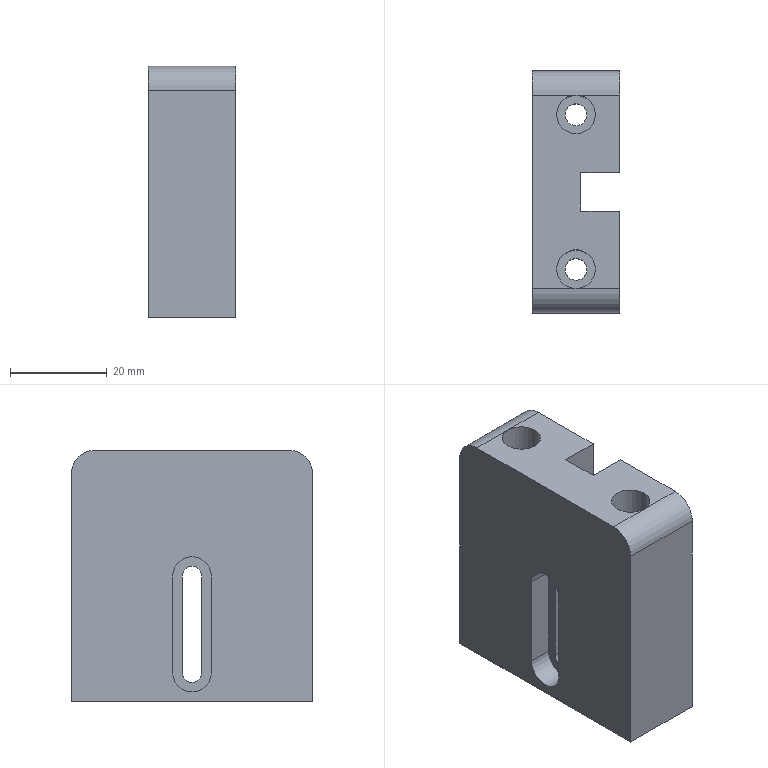Part | SolidWorks | features ICE 2, Extrusion 1, Fillet 1, HoleWzd 1 | 1 solid | 31 faces | box 18 x 50 x 52 mm | volume 37362 mm3 | plane 17 | cylinder 14 | commonest cylinder face diameters 8 x6 4.5 x4 4 x2 10 x2
STEP:
#1=CARTESIAN_POINT('',(-4.,16.,12.));
#2=VERTEX_POINT('',#1);
#3=CARTESIAN_POINT('',(4.,16.,12.));
#4=VERTEX_POINT('',#3);
#5=CARTESIAN_POINT('',(0.,16.,12.));
#6=DIRECTION('',(0.,0.,1.));
#7=DIRECTION('',(1.,0.,0.));
#8=AXIS2_PLACEMENT_3D('',#5,#6,#7);
#9=CIRCLE('',#8,4.);
#10=EDGE_CURVE('',#2,#4,#9,.T.);
#11=ORIENTED_EDGE('',*,*,#10,.F.);
#12=CARTESIAN_POINT('',(-4.,16.,52.));
#13=VERTEX_POINT('',#12);
#14=CARTESIAN_POINT('',(-4.,16.,52.));
#15=DIRECTION('',(0.,0.,1.));
#16=VECTOR('',#15,1000.);
#17=LINE('',#14,#16);
#18=EDGE_CURVE('',#2,#13,#17,.T.);
#19=ORIENTED_EDGE('',*,*,#18,.T.);
#20=CARTESIAN_POINT('',(4.,16.,52.));
#21=VERTEX_POINT('',#20);
#22=CARTESIAN_POINT('',(0.,16.,52.));
#23=DIRECTION('',(0.,0.,1.));
#24=DIRECTION('',(1.,0.,0.));
#25=AXIS2_PLACEMENT_3D('',#22,#23,#24);
#26=CIRCLE('',#25,4.);
#27=EDGE_CURVE('',#13,#21,#26,.T.);
#28=ORIENTED_EDGE('',*,*,#27,.T.);
#29=CARTESIAN_POINT('',(4.,16.,52.));
#30=DIRECTION('',(0.,0.,1.));
#31=VECTOR('',#30,1000.);
#32=LINE('',#29,#31);
#33=EDGE_CURVE('',#4,#21,#32,.T.);
#34=ORIENTED_EDGE('',*,*,#33,.F.);
#35=EDGE_LOOP('',(#11,#19,#28,#34));
#36=FACE_OUTER_BOUND('',#35,.T.);
#37=CARTESIAN_POINT('',(0.,16.,52.));
#38=DIRECTION('',(0.,0.,1.));
#39=DIRECTION('',(1.,0.,0.));
#40=AXIS2_PLACEMENT_3D('',#37,#38,#39);
#41=CYLINDRICAL_SURFACE('',#40,4.);
#42=ADVANCED_FACE('',(#36),#41,.F.);
#43=CARTESIAN_POINT('',(-2.25,16.,0.));
#44=VERTEX_POINT('',#43);
#45=CARTESIAN_POINT('',(2.25,16.,0.));
#46=VERTEX_POINT('',#45);
#47=CARTESIAN_POINT('',(0.,16.,0.));
#48=DIRECTION('',(0.,0.,1.));
#49=DIRECTION('',(1.,0.,0.));
#50=AXIS2_PLACEMENT_3D('',#47,#48,#49);
#51=CIRCLE('',#50,2.25);
#52=EDGE_CURVE('',#44,#46,#51,.T.);
#53=ORIENTED_EDGE('',*,*,#52,.F.);
#54=CARTESIAN_POINT('',(-2.25,16.,12.));
#55=VERTEX_POINT('',#54);
#56=CARTESIAN_POINT('',(-2.25,16.,52.));
#57=DIRECTION('',(0.,0.,1.));
#58=VECTOR('',#57,1000.);
#59=LINE('',#56,#58);
#60=EDGE_CURVE('',#44,#55,#59,.T.);
#61=ORIENTED_EDGE('',*,*,#60,.T.);
#62=CARTESIAN_POINT('',(2.25,16.,12.));
#63=VERTEX_POINT('',#62);
#64=CARTESIAN_POINT('',(0.,16.,12.));
#65=DIRECTION('',(0.,0.,1.));
#66=DIRECTION('',(1.,0.,0.));
#67=AXIS2_PLACEMENT_3D('',#64,#65,#66);
#68=CIRCLE('',#67,2.25);
#69=EDGE_CURVE('',#55,#63,#68,.T.);
#70=ORIENTED_EDGE('',*,*,#69,.T.);
#71=CARTESIAN_POINT('',(2.25,16.,52.));
#72=DIRECTION('',(0.,0.,1.));
#73=VECTOR('',#72,1000.);
#74=LINE('',#71,#73);
#75=EDGE_CURVE('',#46,#63,#74,.T.);
#76=ORIENTED_EDGE('',*,*,#75,.F.);
#77=EDGE_LOOP('',(#53,#61,#70,#76));
#78=FACE_OUTER_BOUND('',#77,.T.);
#79=CARTESIAN_POINT('',(0.,16.,52.));
#80=DIRECTION('',(0.,0.,1.));
#81=DIRECTION('',(1.,0.,0.));
#82=AXIS2_PLACEMENT_3D('',#79,#80,#81);
#83=CYLINDRICAL_SURFACE('',#82,2.25);
#84=ADVANCED_FACE('',(#78),#83,.F.);
#85=CARTESIAN_POINT('',(-4.,-16.,12.));
#86=VERTEX_POINT('',#85);
#87=CARTESIAN_POINT('',(4.,-16.,12.));
#88=VERTEX_POINT('',#87);
#89=CARTESIAN_POINT('',(0.,-16.,12.));
#90=DIRECTION('',(0.,0.,1.));
#91=DIRECTION('',(1.,0.,0.));
#92=AXIS2_PLACEMENT_3D('',#89,#90,#91);
#93=CIRCLE('',#92,4.);
#94=EDGE_CURVE('',#86,#88,#93,.T.);
#95=ORIENTED_EDGE('',*,*,#94,.F.);
#96=CARTESIAN_POINT('',(-4.,-16.,52.));
#97=VERTEX_POINT('',#96);
#98=CARTESIAN_POINT('',(-4.,-16.,52.));
#99=DIRECTION('',(0.,0.,1.));
#100=VECTOR('',#99,1000.);
#101=LINE('',#98,#100);
#102=EDGE_CURVE('',#86,#97,#101,.T.);
#103=ORIENTED_EDGE('',*,*,#102,.T.);
#104=CARTESIAN_POINT('',(0.,-20.,52.));
#105=VERTEX_POINT('',#104);
#106=CARTESIAN_POINT('',(0.,-16.,52.));
#107=DIRECTION('',(0.,0.,1.));
#108=DIRECTION('',(1.,0.,0.));
#109=AXIS2_PLACEMENT_3D('',#106,#107,#108);
#110=CIRCLE('',#109,4.);
#111=EDGE_CURVE('',#97,#105,#110,.T.);
#112=ORIENTED_EDGE('',*,*,#111,.T.);
#113=CARTESIAN_POINT('',(4.,-16.,52.));
#114=VERTEX_POINT('',#113);
#115=CARTESIAN_POINT('',(0.,-16.,52.));
#116=DIRECTION('',(0.,0.,1.));
#117=DIRECTION('',(1.,0.,0.));
#118=AXIS2_PLACEMENT_3D('',#115,#116,#117);
#119=CIRCLE('',#118,4.);
#120=EDGE_CURVE('',#105,#114,#119,.T.);
#121=ORIENTED_EDGE('',*,*,#120,.T.);
#122=CARTESIAN_POINT('',(4.,-16.,52.));
#123=DIRECTION('',(0.,0.,1.));
#124=VECTOR('',#123,1000.);
#125=LINE('',#122,#124);
#126=EDGE_CURVE('',#88,#114,#125,.T.);
#127=ORIENTED_EDGE('',*,*,#126,.F.);
#128=EDGE_LOOP('',(#95,#103,#112,#121,#127));
#129=FACE_OUTER_BOUND('',#128,.T.);
#130=CARTESIAN_POINT('',(0.,-16.,52.));
#131=DIRECTION('',(0.,0.,1.));
#132=DIRECTION('',(1.,0.,0.));
#133=AXIS2_PLACEMENT_3D('',#130,#131,#132);
#134=CYLINDRICAL_SURFACE('',#133,4.);
#135=ADVANCED_FACE('',(#129),#134,.F.);
#136=CARTESIAN_POINT('',(-2.25,-16.,0.));
#137=VERTEX_POINT('',#136);
#138=CARTESIAN_POINT('',(2.25,-16.,0.));
#139=VERTEX_POINT('',#138);
#140=CARTESIAN_POINT('',(0.,-16.,0.));
#141=DIRECTION('',(0.,0.,1.));
#142=DIRECTION('',(1.,0.,0.));
#143=AXIS2_PLACEMENT_3D('',#140,#141,#142);
#144=CIRCLE('',#143,2.25);
#145=EDGE_CURVE('',#137,#139,#144,.T.);
#146=ORIENTED_EDGE('',*,*,#145,.F.);
#147=CARTESIAN_POINT('',(-2.25,-16.,12.));
#148=VERTEX_POINT('',#147);
#149=CARTESIAN_POINT('',(-2.25,-16.,52.));
#150=DIRECTION('',(0.,0.,1.));
#151=VECTOR('',#150,1000.);
#152=LINE('',#149,#151);
#153=EDGE_CURVE('',#137,#148,#152,.T.);
#154=ORIENTED_EDGE('',*,*,#153,.T.);
#155=CARTESIAN_POINT('',(2.25,-16.,12.));
#156=VERTEX_POINT('',#155);
#157=CARTESIAN_POINT('',(0.,-16.,12.));
#158=DIRECTION('',(0.,0.,1.));
#159=DIRECTION('',(1.,0.,0.));
#160=AXIS2_PLACEMENT_3D('',#157,#158,#159);
#161=CIRCLE('',#160,2.25);
#162=EDGE_CURVE('',#148,#156,#161,.T.);
#163=ORIENTED_EDGE('',*,*,#162,.T.);
#164=CARTESIAN_POINT('',(2.25,-16.,52.));
#165=DIRECTION('',(0.,0.,1.));
#166=VECTOR('',#165,1000.);
#167=LINE('',#164,#166);
#168=EDGE_CURVE('',#139,#156,#167,.T.);
#169=ORIENTED_EDGE('',*,*,#168,.F.);
#170=EDGE_LOOP('',(#146,#154,#163,#169));
#171=FACE_OUTER_BOUND('',#170,.T.);
#172=CARTESIAN_POINT('',(0.,-16.,52.));
#173=DIRECTION('',(0.,0.,1.));
#174=DIRECTION('',(1.,0.,0.));
#175=AXIS2_PLACEMENT_3D('',#172,#173,#174);
#176=CYLINDRICAL_SURFACE('',#175,2.25);
#177=ADVANCED_FACE('',(#171),#176,.F.);
#178=CARTESIAN_POINT('',(9.,-25.,47.));
#179=VERTEX_POINT('',#178);
#180=CARTESIAN_POINT('',(9.,-25.,0.));
#181=VERTEX_POINT('',#180);
#182=CARTESIAN_POINT('',(9.,-25.,52.));
#183=DIRECTION('',(0.,0.,-1.));
#184=VECTOR('',#183,1000.);
#185=LINE('',#182,#184);
#186=EDGE_CURVE('',#179,#181,#185,.T.);
#187=ORIENTED_EDGE('',*,*,#186,.F.);
#188=CARTESIAN_POINT('',(-9.,-25.,47.));
#189=VERTEX_POINT('',#188);
#190=CARTESIAN_POINT('',(-9.,-25.,47.));
#191=DIRECTION('',(-1.,0.,0.));
#192=VECTOR('',#191,1000.);
#193=LINE('',#190,#192);
#194=EDGE_CURVE('',#179,#189,#193,.T.);
#195=ORIENTED_EDGE('',*,*,#194,.T.);
#196=CARTESIAN_POINT('',(-9.,-25.,0.));
#197=VERTEX_POINT('',#196);
#198=CARTESIAN_POINT('',(-9.,-25.,52.));
#199=DIRECTION('',(0.,0.,-1.));
#200=VECTOR('',#199,1000.);
#201=LINE('',#198,#200);
#202=EDGE_CURVE('',#189,#197,#201,.T.);
#203=ORIENTED_EDGE('',*,*,#202,.T.);
#204=CARTESIAN_POINT('',(-9.,-25.,0.));
#205=DIRECTION('',(1.,0.,0.));
#206=VECTOR('',#205,1000.);
#207=LINE('',#204,#206);
#208=EDGE_CURVE('',#197,#181,#207,.T.);
#209=ORIENTED_EDGE('',*,*,#208,.T.);
#210=EDGE_LOOP('',(#187,#195,#203,#209));
#211=FACE_OUTER_BOUND('',#210,.T.);
#212=CARTESIAN_POINT('',(-9.,-25.,52.));
#213=DIRECTION('',(0.,1.,0.));
#214=DIRECTION('',(0.,0.,1.));
#215=AXIS2_PLACEMENT_3D('',#212,#213,#214);
#216=PLANE('',#215);
#217=ADVANCED_FACE('',(#211),#216,.F.);
#218=CARTESIAN_POINT('',(9.,-20.,52.));
#219=VERTEX_POINT('',#218);
#220=CARTESIAN_POINT('',(9.,-4.,52.));
#221=VERTEX_POINT('',#220);
#222=CARTESIAN_POINT('',(9.,-4.,52.));
#223=DIRECTION('',(0.,1.,0.));
#224=VECTOR('',#223,1000.);
#225=LINE('',#222,#224);
#226=EDGE_CURVE('',#219,#221,#225,.T.);
#227=ORIENTED_EDGE('',*,*,#226,.F.);
#228=CARTESIAN_POINT('',(9.,-20.,47.));
#229=DIRECTION('',(1.,0.,0.));
#230=DIRECTION('',(0.,-1.,0.));
#231=AXIS2_PLACEMENT_3D('',#228,#229,#230);
#232=CIRCLE('',#231,5.);
#233=EDGE_CURVE('',#219,#179,#232,.T.);
#234=ORIENTED_EDGE('',*,*,#233,.T.);
#235=ORIENTED_EDGE('',*,*,#186,.T.);
#236=CARTESIAN_POINT('',(9.,-4.,0.));
#237=VERTEX_POINT('',#236);
#238=CARTESIAN_POINT('',(9.,-4.,0.));
#239=DIRECTION('',(0.,1.,0.));
#240=VECTOR('',#239,1000.);
#241=LINE('',#238,#240);
#242=EDGE_CURVE('',#181,#237,#241,.T.);
#243=ORIENTED_EDGE('',*,*,#242,.T.);
#244=CARTESIAN_POINT('',(9.,-4.,52.));
#245=DIRECTION('',(0.,0.,-1.));
#246=VECTOR('',#245,1000.);
#247=LINE('',#244,#246);
#248=EDGE_CURVE('',#221,#237,#247,.T.);
#249=ORIENTED_EDGE('',*,*,#248,.F.);
#250=EDGE_LOOP('',(#227,#234,#235,#243,#249));
#251=FACE_OUTER_BOUND('',#250,.T.);
#252=CARTESIAN_POINT('',(9.,-4.,52.));
#253=DIRECTION('',(-1.,0.,0.));
#254=DIRECTION('',(0.,-1.,0.));
#255=AXIS2_PLACEMENT_3D('',#252,#253,#254);
#256=PLANE('',#255);
#257=ADVANCED_FACE('',(#251),#256,.F.);
#258=CARTESIAN_POINT('',(1.,-4.,0.));
#259=VERTEX_POINT('',#258);
#260=CARTESIAN_POINT('',(1.,-4.,0.));
#261=DIRECTION('',(-1.,0.,0.));
#262=VECTOR('',#261,1000.);
#263=LINE('',#260,#262);
#264=EDGE_CURVE('',#237,#259,#263,.T.);
#265=ORIENTED_EDGE('',*,*,#264,.T.);
#266=CARTESIAN_POINT('',(1.,-4.,52.));
#267=VERTEX_POINT('',#266);
#268=CARTESIAN_POINT('',(1.,-4.,52.));
#269=DIRECTION('',(0.,0.,-1.));
#270=VECTOR('',#269,1000.);
#271=LINE('',#268,#270);
#272=EDGE_CURVE('',#267,#259,#271,.T.);
#273=ORIENTED_EDGE('',*,*,#272,.F.);
#274=CARTESIAN_POINT('',(1.,-4.,52.));
#275=DIRECTION('',(-1.,0.,0.));
#276=VECTOR('',#275,1000.);
#277=LINE('',#274,#276);
#278=EDGE_CURVE('',#221,#267,#277,.T.);
#279=ORIENTED_EDGE('',*,*,#278,.F.);
#280=ORIENTED_EDGE('',*,*,#248,.T.);
#281=EDGE_LOOP('',(#265,#273,#279,#280));
#282=FACE_OUTER_BOUND('',#281,.T.);
#283=CARTESIAN_POINT('',(1.,-4.,52.));
#284=DIRECTION('',(0.,-1.,0.));
#285=DIRECTION('',(0.,0.,-1.));
#286=AXIS2_PLACEMENT_3D('',#283,#284,#285);
#287=PLANE('',#286);
#288=ADVANCED_FACE('',(#282),#287,.F.);
#289=CARTESIAN_POINT('',(1.,2.,26.));
#290=VERTEX_POINT('',#289);
#291=CARTESIAN_POINT('',(1.,2.,6.));
#292=VERTEX_POINT('',#291);
#293=CARTESIAN_POINT('',(1.,2.,52.));
#294=DIRECTION('',(0.,0.,-1.));
#295=VECTOR('',#294,1000.);
#296=LINE('',#293,#295);
#297=EDGE_CURVE('',#290,#292,#296,.T.);
#298=ORIENTED_EDGE('',*,*,#297,.T.);
#299=CARTESIAN_POINT('',(1.,-2.,6.));
#300=VERTEX_POINT('',#299);
#301=CARTESIAN_POINT('',(1.,0.,6.));
#302=DIRECTION('',(-1.,0.,0.));
#303=DIRECTION('',(0.,0.,1.));
#304=AXIS2_PLACEMENT_3D('',#301,#302,#303);
#305=CIRCLE('',#304,2.);
#306=EDGE_CURVE('',#292,#300,#305,.T.);
#307=ORIENTED_EDGE('',*,*,#306,.T.);
#308=CARTESIAN_POINT('',(1.,-2.,26.));
#309=VERTEX_POINT('',#308);
#310=CARTESIAN_POINT('',(1.,-2.,52.));
#311=DIRECTION('',(0.,0.,1.));
#312=VECTOR('',#311,1000.);
#313=LINE('',#310,#312);
#314=EDGE_CURVE('',#300,#309,#313,.T.);
#315=ORIENTED_EDGE('',*,*,#314,.T.);
#316=CARTESIAN_POINT('',(1.,0.,26.));
#317=DIRECTION('',(-1.,0.,0.));
#318=DIRECTION('',(0.,0.,1.));
#319=AXIS2_PLACEMENT_3D('',#316,#317,#318);
#320=CIRCLE('',#319,2.);
#321=EDGE_CURVE('',#309,#290,#320,.T.);
#322=ORIENTED_EDGE('',*,*,#321,.T.);
#323=EDGE_LOOP('',(#298,#307,#315,#322));
#324=FACE_BOUND('',#323,.T.);
#325=CARTESIAN_POINT('',(1.,4.,0.));
#326=VERTEX_POINT('',#325);
#327=CARTESIAN_POINT('',(1.,4.,0.));
#328=DIRECTION('',(0.,1.,0.));
#329=VECTOR('',#328,1000.);
#330=LINE('',#327,#329);
#331=EDGE_CURVE('',#259,#326,#330,.T.);
#332=ORIENTED_EDGE('',*,*,#331,.T.);
#333=CARTESIAN_POINT('',(1.,4.,52.));
#334=VERTEX_POINT('',#333);
#335=CARTESIAN_POINT('',(1.,4.,52.));
#336=DIRECTION('',(0.,0.,-1.));
#337=VECTOR('',#336,1000.);
#338=LINE('',#335,#337);
#339=EDGE_CURVE('',#334,#326,#338,.T.);
#340=ORIENTED_EDGE('',*,*,#339,.F.);
#341=CARTESIAN_POINT('',(1.,4.,52.));
#342=DIRECTION('',(0.,1.,0.));
#343=VECTOR('',#342,1000.);
#344=LINE('',#341,#343);
#345=EDGE_CURVE('',#267,#334,#344,.T.);
#346=ORIENTED_EDGE('',*,*,#345,.F.);
#347=ORIENTED_EDGE('',*,*,#272,.T.);
#348=EDGE_LOOP('',(#332,#340,#346,#347));
#349=FACE_OUTER_BOUND('',#348,.T.);
#350=CARTESIAN_POINT('',(1.,4.,52.));
#351=DIRECTION('',(-1.,0.,0.));
#352=DIRECTION('',(0.,0.,1.));
#353=AXIS2_PLACEMENT_3D('',#350,#351,#352);
#354=PLANE('',#353);
#355=ADVANCED_FACE('',(#324,#349),#354,.F.);
#356=CARTESIAN_POINT('',(9.,4.,0.));
#357=VERTEX_POINT('',#356);
#358=CARTESIAN_POINT('',(1.,4.,0.));
#359=DIRECTION('',(1.,0.,0.));
#360=VECTOR('',#359,1000.);
#361=LINE('',#358,#360);
#362=EDGE_CURVE('',#326,#357,#361,.T.);
#363=ORIENTED_EDGE('',*,*,#362,.T.);
#364=CARTESIAN_POINT('',(9.,4.,52.));
#365=VERTEX_POINT('',#364);
#366=CARTESIAN_POINT('',(9.,4.,52.));
#367=DIRECTION('',(0.,0.,-1.));
#368=VECTOR('',#367,1000.);
#369=LINE('',#366,#368);
#370=EDGE_CURVE('',#365,#357,#369,.T.);
#371=ORIENTED_EDGE('',*,*,#370,.F.);
#372=CARTESIAN_POINT('',(1.,4.,52.));
#373=DIRECTION('',(1.,0.,0.));
#374=VECTOR('',#373,1000.);
#375=LINE('',#372,#374);
#376=EDGE_CURVE('',#334,#365,#375,.T.);
#377=ORIENTED_EDGE('',*,*,#376,.F.);
#378=ORIENTED_EDGE('',*,*,#339,.T.);
#379=EDGE_LOOP('',(#363,#371,#377,#378));
#380=FACE_OUTER_BOUND('',#379,.T.);
#381=CARTESIAN_POINT('',(1.,4.,52.));
#382=DIRECTION('',(0.,1.,0.));
#383=DIRECTION('',(0.,0.,1.));
#384=AXIS2_PLACEMENT_3D('',#381,#382,#383);
#385=PLANE('',#384);
#386=ADVANCED_FACE('',(#380),#385,.F.);
#387=CARTESIAN_POINT('',(9.,25.,47.));
#388=VERTEX_POINT('',#387);
#389=CARTESIAN_POINT('',(9.,25.,0.));
#390=VERTEX_POINT('',#389);
#391=CARTESIAN_POINT('',(9.,25.,52.));
#392=DIRECTION('',(0.,0.,-1.));
#393=VECTOR('',#392,1000.);
#394=LINE('',#391,#393);
#395=EDGE_CURVE('',#388,#390,#394,.T.);
#396=ORIENTED_EDGE('',*,*,#395,.F.);
#397=CARTESIAN_POINT('',(9.,20.,52.));
#398=VERTEX_POINT('',#397);
#399=CARTESIAN_POINT('',(9.,20.,47.));
#400=DIRECTION('',(1.,0.,0.));
#401=DIRECTION('',(0.,0.,1.));
#402=AXIS2_PLACEMENT_3D('',#399,#400,#401);
#403=CIRCLE('',#402,5.);
#404=EDGE_CURVE('',#388,#398,#403,.T.);
#405=ORIENTED_EDGE('',*,*,#404,.T.);
#406=CARTESIAN_POINT('',(9.,25.,52.));
#407=DIRECTION('',(0.,1.,0.));
#408=VECTOR('',#407,1000.);
#409=LINE('',#406,#408);
#410=EDGE_CURVE('',#365,#398,#409,.T.);
#411=ORIENTED_EDGE('',*,*,#410,.F.);
#412=ORIENTED_EDGE('',*,*,#370,.T.);
#413=CARTESIAN_POINT('',(9.,25.,0.));
#414=DIRECTION('',(0.,1.,0.));
#415=VECTOR('',#414,1000.);
#416=LINE('',#413,#415);
#417=EDGE_CURVE('',#357,#390,#416,.T.);
#418=ORIENTED_EDGE('',*,*,#417,.T.);
#419=EDGE_LOOP('',(#396,#405,#411,#412,#418));
#420=FACE_OUTER_BOUND('',#419,.T.);
#421=CARTESIAN_POINT('',(9.,25.,52.));
#422=DIRECTION('',(-1.,0.,0.));
#423=DIRECTION('',(0.,0.,1.));
#424=AXIS2_PLACEMENT_3D('',#421,#422,#423);
#425=PLANE('',#424);
#426=ADVANCED_FACE('',(#420),#425,.F.);
#427=CARTESIAN_POINT('',(-9.,25.,47.));
#428=VERTEX_POINT('',#427);
#429=CARTESIAN_POINT('',(-9.,25.,0.));
#430=VERTEX_POINT('',#429);
#431=CARTESIAN_POINT('',(-9.,25.,52.));
#432=DIRECTION('',(0.,0.,-1.));
#433=VECTOR('',#432,1000.);
#434=LINE('',#431,#433);
#435=EDGE_CURVE('',#428,#430,#434,.T.);
#436=ORIENTED_EDGE('',*,*,#435,.F.);
#437=CARTESIAN_POINT('',(-9.,25.,47.));
#438=DIRECTION('',(1.,0.,0.));
#439=VECTOR('',#438,1000.);
#440=LINE('',#437,#439);
#441=EDGE_CURVE('',#428,#388,#440,.T.);
#442=ORIENTED_EDGE('',*,*,#441,.T.);
#443=ORIENTED_EDGE('',*,*,#395,.T.);
#444=CARTESIAN_POINT('',(-9.,25.,0.));
#445=DIRECTION('',(-1.,0.,0.));
#446=VECTOR('',#445,1000.);
#447=LINE('',#444,#446);
#448=EDGE_CURVE('',#390,#430,#447,.T.);
#449=ORIENTED_EDGE('',*,*,#448,.T.);
#450=EDGE_LOOP('',(#436,#442,#443,#449));
#451=FACE_OUTER_BOUND('',#450,.T.);
#452=CARTESIAN_POINT('',(-9.,25.,52.));
#453=DIRECTION('',(0.,-1.,0.));
#454=DIRECTION('',(0.,0.,-1.));
#455=AXIS2_PLACEMENT_3D('',#452,#453,#454);
#456=PLANE('',#455);
#457=ADVANCED_FACE('',(#451),#456,.F.);
#458=CARTESIAN_POINT('',(-9.,-4.,6.));
#459=VERTEX_POINT('',#458);
#460=CARTESIAN_POINT('',(-9.,-4.,26.));
#461=VERTEX_POINT('',#460);
#462=CARTESIAN_POINT('',(-9.,-4.,6.));
#463=DIRECTION('',(0.,0.,1.));
#464=VECTOR('',#463,1000.);
#465=LINE('',#462,#464);
#466=EDGE_CURVE('',#459,#461,#465,.T.);
#467=ORIENTED_EDGE('',*,*,#466,.F.);
#468=CARTESIAN_POINT('',(-9.,4.,6.));
#469=VERTEX_POINT('',#468);
#470=CARTESIAN_POINT('',(-9.,0.,6.));
#471=DIRECTION('',(-1.,0.,0.));
#472=DIRECTION('',(0.,-1.,0.));
#473=AXIS2_PLACEMENT_3D('',#470,#471,#472);
#474=CIRCLE('',#473,4.);
#475=EDGE_CURVE('',#469,#459,#474,.T.);
#476=ORIENTED_EDGE('',*,*,#475,.F.);
#477=CARTESIAN_POINT('',(-9.,4.,26.));
#478=VERTEX_POINT('',#477);
#479=CARTESIAN_POINT('',(-9.,4.,6.));
#480=DIRECTION('',(0.,0.,-1.));
#481=VECTOR('',#480,1000.);
#482=LINE('',#479,#481);
#483=EDGE_CURVE('',#478,#469,#482,.T.);
#484=ORIENTED_EDGE('',*,*,#483,.F.);
#485=CARTESIAN_POINT('',(-9.,0.,26.));
#486=DIRECTION('',(-1.,0.,0.));
#487=DIRECTION('',(0.,-1.,0.));
#488=AXIS2_PLACEMENT_3D('',#485,#486,#487);
#489=CIRCLE('',#488,4.);
#490=EDGE_CURVE('',#461,#478,#489,.T.);
#491=ORIENTED_EDGE('',*,*,#490,.F.);
#492=EDGE_LOOP('',(#467,#476,#484,#491));
#493=FACE_BOUND('',#492,.T.);
#494=CARTESIAN_POINT('',(-9.,20.,52.));
#495=VERTEX_POINT('',#494);
#496=CARTESIAN_POINT('',(-9.,-20.,52.));
#497=VERTEX_POINT('',#496);
#498=CARTESIAN_POINT('',(-9.,25.,52.));
#499=DIRECTION('',(0.,-1.,0.));
#500=VECTOR('',#499,1000.);
#501=LINE('',#498,#500);
#502=EDGE_CURVE('',#495,#497,#501,.T.);
#503=ORIENTED_EDGE('',*,*,#502,.F.);
#504=CARTESIAN_POINT('',(-9.,20.,47.));
#505=DIRECTION('',(-1.,0.,0.));
#506=DIRECTION('',(0.,1.,0.));
#507=AXIS2_PLACEMENT_3D('',#504,#505,#506);
#508=CIRCLE('',#507,5.);
#509=EDGE_CURVE('',#495,#428,#508,.T.);
#510=ORIENTED_EDGE('',*,*,#509,.T.);
#511=ORIENTED_EDGE('',*,*,#435,.T.);
#512=CARTESIAN_POINT('',(-9.,25.,0.));
#513=DIRECTION('',(0.,-1.,0.));
#514=VECTOR('',#513,1000.);
#515=LINE('',#512,#514);
#516=EDGE_CURVE('',#430,#197,#515,.T.);
#517=ORIENTED_EDGE('',*,*,#516,.T.);
#518=ORIENTED_EDGE('',*,*,#202,.F.);
#519=CARTESIAN_POINT('',(-9.,-20.,47.));
#520=DIRECTION('',(-1.,0.,0.));
#521=DIRECTION('',(0.,1.,0.));
#522=AXIS2_PLACEMENT_3D('',#519,#520,#521);
#523=CIRCLE('',#522,5.);
#524=EDGE_CURVE('',#189,#497,#523,.T.);
#525=ORIENTED_EDGE('',*,*,#524,.T.);
#526=EDGE_LOOP('',(#503,#510,#511,#517,#518,#525));
#527=FACE_OUTER_BOUND('',#526,.T.);
#528=CARTESIAN_POINT('',(-9.,25.,52.));
#529=DIRECTION('',(1.,0.,0.));
#530=DIRECTION('',(0.,1.,0.));
#531=AXIS2_PLACEMENT_3D('',#528,#529,#530);
#532=PLANE('',#531);
#533=ADVANCED_FACE('',(#493,#527),#532,.F.);
#534=ORIENTED_EDGE('',*,*,#410,.T.);
#535=CARTESIAN_POINT('',(0.,20.,52.));
#536=VERTEX_POINT('',#535);
#537=CARTESIAN_POINT('',(0.,20.,52.));
#538=DIRECTION('',(-1.,0.,0.));
#539=VECTOR('',#538,1000.);
#540=LINE('',#537,#539);
#541=EDGE_CURVE('',#398,#536,#540,.T.);
#542=ORIENTED_EDGE('',*,*,#541,.T.);
#543=CARTESIAN_POINT('',(0.,16.,52.));
#544=DIRECTION('',(0.,0.,1.));
#545=DIRECTION('',(1.,0.,0.));
#546=AXIS2_PLACEMENT_3D('',#543,#544,#545);
#547=CIRCLE('',#546,4.);
#548=EDGE_CURVE('',#21,#536,#547,.T.);
#549=ORIENTED_EDGE('',*,*,#548,.F.);
#550=ORIENTED_EDGE('',*,*,#27,.F.);
#551=CARTESIAN_POINT('',(0.,16.,52.));
#552=DIRECTION('',(0.,0.,1.));
#553=DIRECTION('',(1.,0.,0.));
#554=AXIS2_PLACEMENT_3D('',#551,#552,#553);
#555=CIRCLE('',#554,4.);
#556=EDGE_CURVE('',#536,#13,#555,.T.);
#557=ORIENTED_EDGE('',*,*,#556,.F.);
#558=CARTESIAN_POINT('',(0.,20.,52.));
#559=DIRECTION('',(-1.,0.,0.));
#560=VECTOR('',#559,1000.);
#561=LINE('',#558,#560);
#562=EDGE_CURVE('',#536,#495,#561,.T.);
#563=ORIENTED_EDGE('',*,*,#562,.T.);
#564=ORIENTED_EDGE('',*,*,#502,.T.);
#565=CARTESIAN_POINT('',(0.,-20.,52.));
#566=DIRECTION('',(1.,0.,0.));
#567=VECTOR('',#566,1000.);
#568=LINE('',#565,#567);
#569=EDGE_CURVE('',#497,#105,#568,.T.);
#570=ORIENTED_EDGE('',*,*,#569,.T.);
#571=ORIENTED_EDGE('',*,*,#111,.F.);
#572=CARTESIAN_POINT('',(0.,-16.,52.));
#573=DIRECTION('',(0.,0.,1.));
#574=DIRECTION('',(1.,0.,0.));
#575=AXIS2_PLACEMENT_3D('',#572,#573,#574);
#576=CIRCLE('',#575,4.);
#577=EDGE_CURVE('',#114,#97,#576,.T.);
#578=ORIENTED_EDGE('',*,*,#577,.F.);
#579=ORIENTED_EDGE('',*,*,#120,.F.);
#580=CARTESIAN_POINT('',(0.,-20.,52.));
#581=DIRECTION('',(1.,0.,0.));
#582=VECTOR('',#581,1000.);
#583=LINE('',#580,#582);
#584=EDGE_CURVE('',#105,#219,#583,.T.);
#585=ORIENTED_EDGE('',*,*,#584,.T.);
#586=ORIENTED_EDGE('',*,*,#226,.T.);
#587=ORIENTED_EDGE('',*,*,#278,.T.);
#588=ORIENTED_EDGE('',*,*,#345,.T.);
#589=ORIENTED_EDGE('',*,*,#376,.T.);
#590=EDGE_LOOP('',(#534,#542,#549,#550,#557,#563,#564,#570,#571,#578,#579,#585,#586,#587,#588,#589));
#591=FACE_OUTER_BOUND('',#590,.T.);
#592=CARTESIAN_POINT('',(0.,0.,52.));
#593=DIRECTION('',(0.,0.,-1.));
#594=DIRECTION('',(-1.,0.,0.));
#595=AXIS2_PLACEMENT_3D('',#592,#593,#594);
#596=PLANE('',#595);
#597=ADVANCED_FACE('',(#591),#596,.F.);
#598=CARTESIAN_POINT('',(0.,16.,0.));
#599=DIRECTION('',(0.,0.,1.));
#600=DIRECTION('',(1.,0.,0.));
#601=AXIS2_PLACEMENT_3D('',#598,#599,#600);
#602=CIRCLE('',#601,2.25);
#603=EDGE_CURVE('',#46,#44,#602,.T.);
#604=ORIENTED_EDGE('',*,*,#603,.T.);
#605=ORIENTED_EDGE('',*,*,#52,.T.);
#606=EDGE_LOOP('',(#604,#605));
#607=FACE_BOUND('',#606,.T.);
#608=CARTESIAN_POINT('',(0.,-16.,0.));
#609=DIRECTION('',(0.,0.,1.));
#610=DIRECTION('',(1.,0.,0.));
#611=AXIS2_PLACEMENT_3D('',#608,#609,#610);
#612=CIRCLE('',#611,2.25);
#613=EDGE_CURVE('',#139,#137,#612,.T.);
#614=ORIENTED_EDGE('',*,*,#613,.T.);
#615=ORIENTED_EDGE('',*,*,#145,.T.);
#616=EDGE_LOOP('',(#614,#615));
#617=FACE_BOUND('',#616,.T.);
#618=ORIENTED_EDGE('',*,*,#208,.F.);
#619=ORIENTED_EDGE('',*,*,#516,.F.);
#620=ORIENTED_EDGE('',*,*,#448,.F.);
#621=ORIENTED_EDGE('',*,*,#417,.F.);
#622=ORIENTED_EDGE('',*,*,#362,.F.);
#623=ORIENTED_EDGE('',*,*,#331,.F.);
#624=ORIENTED_EDGE('',*,*,#264,.F.);
#625=ORIENTED_EDGE('',*,*,#242,.F.);
#626=EDGE_LOOP('',(#618,#619,#620,#621,#622,#623,#624,#625));
#627=FACE_OUTER_BOUND('',#626,.T.);
#628=CARTESIAN_POINT('',(0.,0.,0.));
#629=DIRECTION('',(0.,0.,-1.));
#630=DIRECTION('',(-1.,0.,0.));
#631=AXIS2_PLACEMENT_3D('',#628,#629,#630);
#632=PLANE('',#631);
#633=ADVANCED_FACE('',(#607,#617,#627),#632,.T.);
#634=ORIENTED_EDGE('',*,*,#153,.F.);
#635=ORIENTED_EDGE('',*,*,#613,.F.);
#636=ORIENTED_EDGE('',*,*,#168,.T.);
#637=CARTESIAN_POINT('',(0.,-16.,12.));
#638=DIRECTION('',(0.,0.,1.));
#639=DIRECTION('',(1.,0.,0.));
#640=AXIS2_PLACEMENT_3D('',#637,#638,#639);
#641=CIRCLE('',#640,2.25);
#642=EDGE_CURVE('',#156,#148,#641,.T.);
#643=ORIENTED_EDGE('',*,*,#642,.T.);
#644=EDGE_LOOP('',(#634,#635,#636,#643));
#645=FACE_OUTER_BOUND('',#644,.T.);
#646=CARTESIAN_POINT('',(0.,-16.,52.));
#647=DIRECTION('',(0.,0.,1.));
#648=DIRECTION('',(1.,0.,0.));
#649=AXIS2_PLACEMENT_3D('',#646,#647,#648);
#650=CYLINDRICAL_SURFACE('',#649,2.25);
#651=ADVANCED_FACE('',(#645),#650,.F.);
#652=ORIENTED_EDGE('',*,*,#642,.F.);
#653=ORIENTED_EDGE('',*,*,#162,.F.);
#654=EDGE_LOOP('',(#652,#653));
#655=FACE_BOUND('',#654,.T.);
#656=CARTESIAN_POINT('',(0.,-16.,12.));
#657=DIRECTION('',(0.,0.,1.));
#658=DIRECTION('',(1.,0.,0.));
#659=AXIS2_PLACEMENT_3D('',#656,#657,#658);
#660=CIRCLE('',#659,4.);
#661=EDGE_CURVE('',#88,#86,#660,.T.);
#662=ORIENTED_EDGE('',*,*,#661,.T.);
#663=ORIENTED_EDGE('',*,*,#94,.T.);
#664=EDGE_LOOP('',(#662,#663));
#665=FACE_OUTER_BOUND('',#664,.T.);
#666=CARTESIAN_POINT('',(2.25,-16.,12.));
#667=DIRECTION('',(0.,0.,-1.));
#668=DIRECTION('',(-1.,0.,0.));
#669=AXIS2_PLACEMENT_3D('',#666,#667,#668);
#670=PLANE('',#669);
#671=ADVANCED_FACE('',(#655,#665),#670,.F.);
#672=ORIENTED_EDGE('',*,*,#102,.F.);
#673=ORIENTED_EDGE('',*,*,#661,.F.);
#674=ORIENTED_EDGE('',*,*,#126,.T.);
#675=ORIENTED_EDGE('',*,*,#577,.T.);
#676=EDGE_LOOP('',(#672,#673,#674,#675));
#677=FACE_OUTER_BOUND('',#676,.T.);
#678=CARTESIAN_POINT('',(0.,-16.,52.));
#679=DIRECTION('',(0.,0.,1.));
#680=DIRECTION('',(1.,0.,0.));
#681=AXIS2_PLACEMENT_3D('',#678,#679,#680);
#682=CYLINDRICAL_SURFACE('',#681,4.);
#683=ADVANCED_FACE('',(#677),#682,.F.);
#684=ORIENTED_EDGE('',*,*,#60,.F.);
#685=ORIENTED_EDGE('',*,*,#603,.F.);
#686=ORIENTED_EDGE('',*,*,#75,.T.);
#687=CARTESIAN_POINT('',(0.,16.,12.));
#688=DIRECTION('',(0.,0.,1.));
#689=DIRECTION('',(1.,0.,0.));
#690=AXIS2_PLACEMENT_3D('',#687,#688,#689);
#691=CIRCLE('',#690,2.25);
#692=EDGE_CURVE('',#63,#55,#691,.T.);
#693=ORIENTED_EDGE('',*,*,#692,.T.);
#694=EDGE_LOOP('',(#684,#685,#686,#693));
#695=FACE_OUTER_BOUND('',#694,.T.);
#696=CARTESIAN_POINT('',(0.,16.,52.));
#697=DIRECTION('',(0.,0.,1.));
#698=DIRECTION('',(1.,0.,0.));
#699=AXIS2_PLACEMENT_3D('',#696,#697,#698);
#700=CYLINDRICAL_SURFACE('',#699,2.25);
#701=ADVANCED_FACE('',(#695),#700,.F.);
#702=ORIENTED_EDGE('',*,*,#692,.F.);
#703=ORIENTED_EDGE('',*,*,#69,.F.);
#704=EDGE_LOOP('',(#702,#703));
#705=FACE_BOUND('',#704,.T.);
#706=CARTESIAN_POINT('',(0.,16.,12.));
#707=DIRECTION('',(0.,0.,1.));
#708=DIRECTION('',(1.,0.,0.));
#709=AXIS2_PLACEMENT_3D('',#706,#707,#708);
#710=CIRCLE('',#709,4.);
#711=EDGE_CURVE('',#4,#2,#710,.T.);
#712=ORIENTED_EDGE('',*,*,#711,.T.);
#713=ORIENTED_EDGE('',*,*,#10,.T.);
#714=EDGE_LOOP('',(#712,#713));
#715=FACE_OUTER_BOUND('',#714,.T.);
#716=CARTESIAN_POINT('',(2.25,16.,12.));
#717=DIRECTION('',(0.,0.,-1.));
#718=DIRECTION('',(-1.,0.,0.));
#719=AXIS2_PLACEMENT_3D('',#716,#717,#718);
#720=PLANE('',#719);
#721=ADVANCED_FACE('',(#705,#715),#720,.F.);
#722=ORIENTED_EDGE('',*,*,#18,.F.);
#723=ORIENTED_EDGE('',*,*,#711,.F.);
#724=ORIENTED_EDGE('',*,*,#33,.T.);
#725=ORIENTED_EDGE('',*,*,#548,.T.);
#726=ORIENTED_EDGE('',*,*,#556,.T.);
#727=EDGE_LOOP('',(#722,#723,#724,#725,#726));
#728=FACE_OUTER_BOUND('',#727,.T.);
#729=CARTESIAN_POINT('',(0.,16.,52.));
#730=DIRECTION('',(0.,0.,1.));
#731=DIRECTION('',(1.,0.,0.));
#732=AXIS2_PLACEMENT_3D('',#729,#730,#731);
#733=CYLINDRICAL_SURFACE('',#732,4.);
#734=ADVANCED_FACE('',(#728),#733,.F.);
#735=ORIENTED_EDGE('',*,*,#404,.F.);
#736=ORIENTED_EDGE('',*,*,#441,.F.);
#737=ORIENTED_EDGE('',*,*,#509,.F.);
#738=ORIENTED_EDGE('',*,*,#562,.F.);
#739=ORIENTED_EDGE('',*,*,#541,.F.);
#740=EDGE_LOOP('',(#735,#736,#737,#738,#739));
#741=FACE_OUTER_BOUND('',#740,.T.);
#742=CARTESIAN_POINT('',(0.,20.,47.));
#743=DIRECTION('',(-1.,0.,0.));
#744=DIRECTION('',(0.,0.,1.));
#745=AXIS2_PLACEMENT_3D('',#742,#743,#744);
#746=CYLINDRICAL_SURFACE('',#745,5.);
#747=ADVANCED_FACE('',(#741),#746,.T.);
#748=ORIENTED_EDGE('',*,*,#524,.F.);
#749=ORIENTED_EDGE('',*,*,#194,.F.);
#750=ORIENTED_EDGE('',*,*,#233,.F.);
#751=ORIENTED_EDGE('',*,*,#584,.F.);
#752=ORIENTED_EDGE('',*,*,#569,.F.);
#753=EDGE_LOOP('',(#748,#749,#750,#751,#752));
#754=FACE_OUTER_BOUND('',#753,.T.);
#755=CARTESIAN_POINT('',(0.,-20.,47.));
#756=DIRECTION('',(1.,0.,0.));
#757=DIRECTION('',(0.,0.,-1.));
#758=AXIS2_PLACEMENT_3D('',#755,#756,#757);
#759=CYLINDRICAL_SURFACE('',#758,5.);
#760=ADVANCED_FACE('',(#754),#759,.T.);
#761=ORIENTED_EDGE('',*,*,#475,.T.);
#762=CARTESIAN_POINT('',(-4.,-4.,6.));
#763=VERTEX_POINT('',#762);
#764=CARTESIAN_POINT('',(-4.,-4.,6.));
#765=DIRECTION('',(-1.,0.,0.));
#766=VECTOR('',#765,1000.);
#767=LINE('',#764,#766);
#768=EDGE_CURVE('',#763,#459,#767,.T.);
#769=ORIENTED_EDGE('',*,*,#768,.F.);
#770=CARTESIAN_POINT('',(-4.,4.,6.));
#771=VERTEX_POINT('',#770);
#772=CARTESIAN_POINT('',(-4.,0.,6.));
#773=DIRECTION('',(-1.,0.,0.));
#774=DIRECTION('',(0.,-1.,0.));
#775=AXIS2_PLACEMENT_3D('',#772,#773,#774);
#776=CIRCLE('',#775,4.);
#777=EDGE_CURVE('',#771,#763,#776,.T.);
#778=ORIENTED_EDGE('',*,*,#777,.F.);
#779=CARTESIAN_POINT('',(-4.,4.,6.));
#780=DIRECTION('',(-1.,0.,0.));
#781=VECTOR('',#780,1000.);
#782=LINE('',#779,#781);
#783=EDGE_CURVE('',#771,#469,#782,.T.);
#784=ORIENTED_EDGE('',*,*,#783,.T.);
#785=EDGE_LOOP('',(#761,#769,#778,#784));
#786=FACE_OUTER_BOUND('',#785,.T.);
#787=CARTESIAN_POINT('',(-4.,0.,6.));
#788=DIRECTION('',(-1.,0.,0.));
#789=DIRECTION('',(0.,-1.,0.));
#790=AXIS2_PLACEMENT_3D('',#787,#788,#789);
#791=CYLINDRICAL_SURFACE('',#790,4.);
#792=ADVANCED_FACE('',(#786),#791,.F.);
#793=ORIENTED_EDGE('',*,*,#483,.T.);
#794=ORIENTED_EDGE('',*,*,#783,.F.);
#795=CARTESIAN_POINT('',(-4.,4.,26.));
#796=VERTEX_POINT('',#795);
#797=CARTESIAN_POINT('',(-4.,4.,6.));
#798=DIRECTION('',(0.,0.,-1.));
#799=VECTOR('',#798,1000.);
#800=LINE('',#797,#799);
#801=EDGE_CURVE('',#796,#771,#800,.T.);
#802=ORIENTED_EDGE('',*,*,#801,.F.);
#803=CARTESIAN_POINT('',(-4.,4.,26.));
#804=DIRECTION('',(-1.,0.,0.));
#805=VECTOR('',#804,1000.);
#806=LINE('',#803,#805);
#807=EDGE_CURVE('',#796,#478,#806,.T.);
#808=ORIENTED_EDGE('',*,*,#807,.T.);
#809=EDGE_LOOP('',(#793,#794,#802,#808));
#810=FACE_OUTER_BOUND('',#809,.T.);
#811=CARTESIAN_POINT('',(-4.,4.,6.));
#812=DIRECTION('',(0.,1.,0.));
#813=DIRECTION('',(-1.,0.,0.));
#814=AXIS2_PLACEMENT_3D('',#811,#812,#813);
#815=PLANE('',#814);
#816=ADVANCED_FACE('',(#810),#815,.F.);
#817=ORIENTED_EDGE('',*,*,#490,.T.);
#818=ORIENTED_EDGE('',*,*,#807,.F.);
#819=CARTESIAN_POINT('',(-4.,-4.,26.));
#820=VERTEX_POINT('',#819);
#821=CARTESIAN_POINT('',(-4.,0.,26.));
#822=DIRECTION('',(-1.,0.,0.));
#823=DIRECTION('',(0.,-1.,0.));
#824=AXIS2_PLACEMENT_3D('',#821,#822,#823);
#825=CIRCLE('',#824,4.);
#826=EDGE_CURVE('',#820,#796,#825,.T.);
#827=ORIENTED_EDGE('',*,*,#826,.F.);
#828=CARTESIAN_POINT('',(-4.,-4.,26.));
#829=DIRECTION('',(-1.,0.,0.));
#830=VECTOR('',#829,1000.);
#831=LINE('',#828,#830);
#832=EDGE_CURVE('',#820,#461,#831,.T.);
#833=ORIENTED_EDGE('',*,*,#832,.T.);
#834=EDGE_LOOP('',(#817,#818,#827,#833));
#835=FACE_OUTER_BOUND('',#834,.T.);
#836=CARTESIAN_POINT('',(-4.,0.,26.));
#837=DIRECTION('',(-1.,0.,0.));
#838=DIRECTION('',(0.,-1.,0.));
#839=AXIS2_PLACEMENT_3D('',#836,#837,#838);
#840=CYLINDRICAL_SURFACE('',#839,4.);
#841=ADVANCED_FACE('',(#835),#840,.F.);
#842=ORIENTED_EDGE('',*,*,#466,.T.);
#843=ORIENTED_EDGE('',*,*,#832,.F.);
#844=CARTESIAN_POINT('',(-4.,-4.,6.));
#845=DIRECTION('',(0.,0.,1.));
#846=VECTOR('',#845,1000.);
#847=LINE('',#844,#846);
#848=EDGE_CURVE('',#763,#820,#847,.T.);
#849=ORIENTED_EDGE('',*,*,#848,.F.);
#850=ORIENTED_EDGE('',*,*,#768,.T.);
#851=EDGE_LOOP('',(#842,#843,#849,#850));
#852=FACE_OUTER_BOUND('',#851,.T.);
#853=CARTESIAN_POINT('',(-4.,-4.,6.));
#854=DIRECTION('',(0.,-1.,0.));
#855=DIRECTION('',(1.,0.,0.));
#856=AXIS2_PLACEMENT_3D('',#853,#854,#855);
#857=PLANE('',#856);
#858=ADVANCED_FACE('',(#852),#857,.F.);
#859=CARTESIAN_POINT('',(-4.,2.,6.));
#860=VERTEX_POINT('',#859);
#861=CARTESIAN_POINT('',(-4.,-2.,6.));
#862=VERTEX_POINT('',#861);
#863=CARTESIAN_POINT('',(-4.,0.,6.));
#864=DIRECTION('',(-1.,0.,0.));
#865=DIRECTION('',(0.,-1.,0.));
#866=AXIS2_PLACEMENT_3D('',#863,#864,#865);
#867=CIRCLE('',#866,2.);
#868=EDGE_CURVE('',#860,#862,#867,.T.);
#869=ORIENTED_EDGE('',*,*,#868,.F.);
#870=CARTESIAN_POINT('',(-4.,2.,26.));
#871=VERTEX_POINT('',#870);
#872=CARTESIAN_POINT('',(-4.,2.,6.));
#873=DIRECTION('',(0.,0.,-1.));
#874=VECTOR('',#873,1000.);
#875=LINE('',#872,#874);
#876=EDGE_CURVE('',#871,#860,#875,.T.);
#877=ORIENTED_EDGE('',*,*,#876,.F.);
#878=CARTESIAN_POINT('',(-4.,-2.,26.));
#879=VERTEX_POINT('',#878);
#880=CARTESIAN_POINT('',(-4.,0.,26.));
#881=DIRECTION('',(-1.,0.,0.));
#882=DIRECTION('',(0.,-1.,0.));
#883=AXIS2_PLACEMENT_3D('',#880,#881,#882);
#884=CIRCLE('',#883,2.);
#885=EDGE_CURVE('',#879,#871,#884,.T.);
#886=ORIENTED_EDGE('',*,*,#885,.F.);
#887=CARTESIAN_POINT('',(-4.,-2.,6.));
#888=DIRECTION('',(0.,0.,1.));
#889=VECTOR('',#888,1000.);
#890=LINE('',#887,#889);
#891=EDGE_CURVE('',#862,#879,#890,.T.);
#892=ORIENTED_EDGE('',*,*,#891,.F.);
#893=EDGE_LOOP('',(#869,#877,#886,#892));
#894=FACE_BOUND('',#893,.T.);
#895=ORIENTED_EDGE('',*,*,#777,.T.);
#896=ORIENTED_EDGE('',*,*,#848,.T.);
#897=ORIENTED_EDGE('',*,*,#826,.T.);
#898=ORIENTED_EDGE('',*,*,#801,.T.);
#899=EDGE_LOOP('',(#895,#896,#897,#898));
#900=FACE_OUTER_BOUND('',#899,.T.);
#901=CARTESIAN_POINT('',(-4.,0.,6.));
#902=DIRECTION('',(-1.,0.,0.));
#903=DIRECTION('',(0.,-1.,0.));
#904=AXIS2_PLACEMENT_3D('',#901,#902,#903);
#905=PLANE('',#904);
#906=ADVANCED_FACE('',(#894,#900),#905,.T.);
#907=CARTESIAN_POINT('',(9.,2.,6.));
#908=DIRECTION('',(-1.,0.,0.));
#909=VECTOR('',#908,1000.);
#910=LINE('',#907,#909);
#911=EDGE_CURVE('',#292,#860,#910,.T.);
#912=ORIENTED_EDGE('',*,*,#911,.T.);
#913=ORIENTED_EDGE('',*,*,#868,.T.);
#914=CARTESIAN_POINT('',(9.,-2.,6.));
#915=DIRECTION('',(-1.,0.,0.));
#916=VECTOR('',#915,1000.);
#917=LINE('',#914,#916);
#918=EDGE_CURVE('',#300,#862,#917,.T.);
#919=ORIENTED_EDGE('',*,*,#918,.F.);
#920=ORIENTED_EDGE('',*,*,#306,.F.);
#921=EDGE_LOOP('',(#912,#913,#919,#920));
#922=FACE_OUTER_BOUND('',#921,.T.);
#923=CARTESIAN_POINT('',(9.,0.,6.));
#924=DIRECTION('',(-1.,0.,0.));
#925=DIRECTION('',(0.,-1.,0.));
#926=AXIS2_PLACEMENT_3D('',#923,#924,#925);
#927=CYLINDRICAL_SURFACE('',#926,2.);
#928=ADVANCED_FACE('',(#922),#927,.F.);
#929=CARTESIAN_POINT('',(9.,2.,26.));
#930=DIRECTION('',(-1.,0.,0.));
#931=VECTOR('',#930,1000.);
#932=LINE('',#929,#931);
#933=EDGE_CURVE('',#290,#871,#932,.T.);
#934=ORIENTED_EDGE('',*,*,#933,.T.);
#935=ORIENTED_EDGE('',*,*,#876,.T.);
#936=ORIENTED_EDGE('',*,*,#911,.F.);
#937=ORIENTED_EDGE('',*,*,#297,.F.);
#938=EDGE_LOOP('',(#934,#935,#936,#937));
#939=FACE_OUTER_BOUND('',#938,.T.);
#940=CARTESIAN_POINT('',(9.,2.,6.));
#941=DIRECTION('',(0.,1.,0.));
#942=DIRECTION('',(-1.,0.,0.));
#943=AXIS2_PLACEMENT_3D('',#940,#941,#942);
#944=PLANE('',#943);
#945=ADVANCED_FACE('',(#939),#944,.F.);
#946=CARTESIAN_POINT('',(9.,-2.,26.));
#947=DIRECTION('',(-1.,0.,0.));
#948=VECTOR('',#947,1000.);
#949=LINE('',#946,#948);
#950=EDGE_CURVE('',#309,#879,#949,.T.);
#951=ORIENTED_EDGE('',*,*,#950,.T.);
#952=ORIENTED_EDGE('',*,*,#885,.T.);
#953=ORIENTED_EDGE('',*,*,#933,.F.);
#954=ORIENTED_EDGE('',*,*,#321,.F.);
#955=EDGE_LOOP('',(#951,#952,#953,#954));
#956=FACE_OUTER_BOUND('',#955,.T.);
#957=CARTESIAN_POINT('',(9.,0.,26.));
#958=DIRECTION('',(-1.,0.,0.));
#959=DIRECTION('',(0.,-1.,0.));
#960=AXIS2_PLACEMENT_3D('',#957,#958,#959);
#961=CYLINDRICAL_SURFACE('',#960,2.);
#962=ADVANCED_FACE('',(#956),#961,.F.);
#963=ORIENTED_EDGE('',*,*,#918,.T.);
#964=ORIENTED_EDGE('',*,*,#891,.T.);
#965=ORIENTED_EDGE('',*,*,#950,.F.);
#966=ORIENTED_EDGE('',*,*,#314,.F.);
#967=EDGE_LOOP('',(#963,#964,#965,#966));
#968=FACE_OUTER_BOUND('',#967,.T.);
#969=CARTESIAN_POINT('',(9.,-2.,6.));
#970=DIRECTION('',(0.,-1.,0.));
#971=DIRECTION('',(1.,0.,0.));
#972=AXIS2_PLACEMENT_3D('',#969,#970,#971);
#973=PLANE('',#972);
#974=ADVANCED_FACE('',(#968),#973,.F.);
#975=CLOSED_SHELL('',(#42,#84,#135,#177,#217,#257,#288,#355,#386,#426,#457,#533,#597,#633,#651,#671,#683,#701,#721,#734,#747,#760,#792,#816,#841,#858,#906,#928,#945,#962,#974));
#976=MANIFOLD_SOLID_BREP('',#975);
#977=CARTESIAN_POINT('',(0.,0.,0.));
#978=DIRECTION('',(0.,0.,1.));
#979=DIRECTION('',(1.,0.,0.));
#980=AXIS2_PLACEMENT_3D('',#977,#978,#979);
#981=(LENGTH_UNIT()NAMED_UNIT(*)SI_UNIT(.MILLI.,.METRE.));
#982=UNCERTAINTY_MEASURE_WITH_UNIT(LENGTH_MEASURE(0.00001),#981,'','');
#983=(NAMED_UNIT(*)PLANE_ANGLE_UNIT()SI_UNIT($,.RADIAN.));
#984=(NAMED_UNIT(*)SI_UNIT($,.STERADIAN.)SOLID_ANGLE_UNIT());
#985=(GEOMETRIC_REPRESENTATION_CONTEXT(3)GLOBAL_UNCERTAINTY_ASSIGNED_CONTEXT((#982))GLOBAL_UNIT_ASSIGNED_CONTEXT((#981,#983,#984))REPRESENTATION_CONTEXT('',''));
#986=ADVANCED_BREP_SHAPE_REPRESENTATION('',(#976,#980),#985);